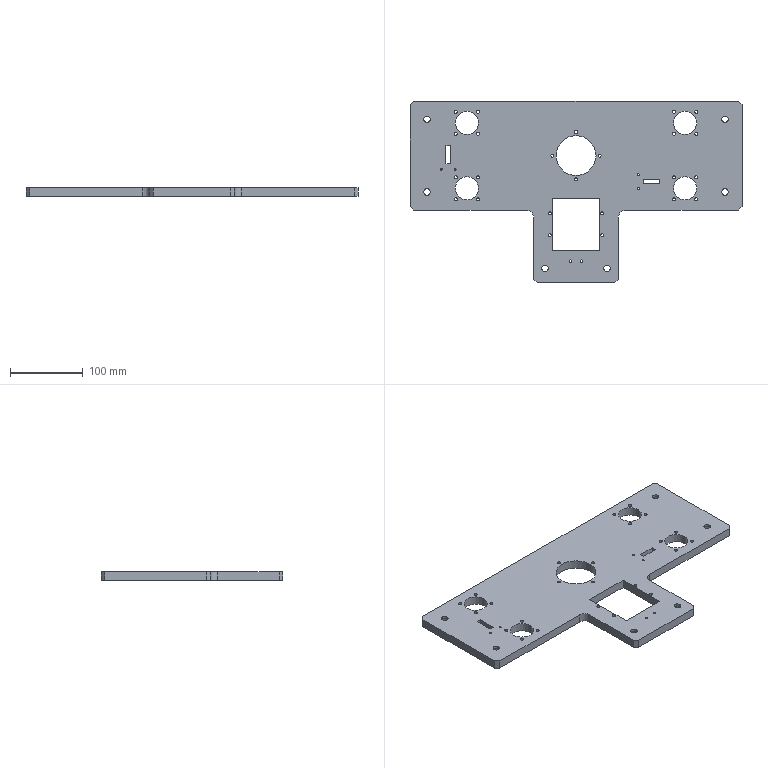Part | SolidWorks | features HoleWzd 6, ICE 5, Chamfer 1, Extrusion 1, Fillet 1 | 1 solid | 130 faces | box 456.5 x 250 x 12 mm | volume 820390 mm3 | cylinder 96 | plane 34 | commonest cylinder face diameters 4.2 x48 9 x12 15 x12 2.5 x8 32 x8 3.3 x4